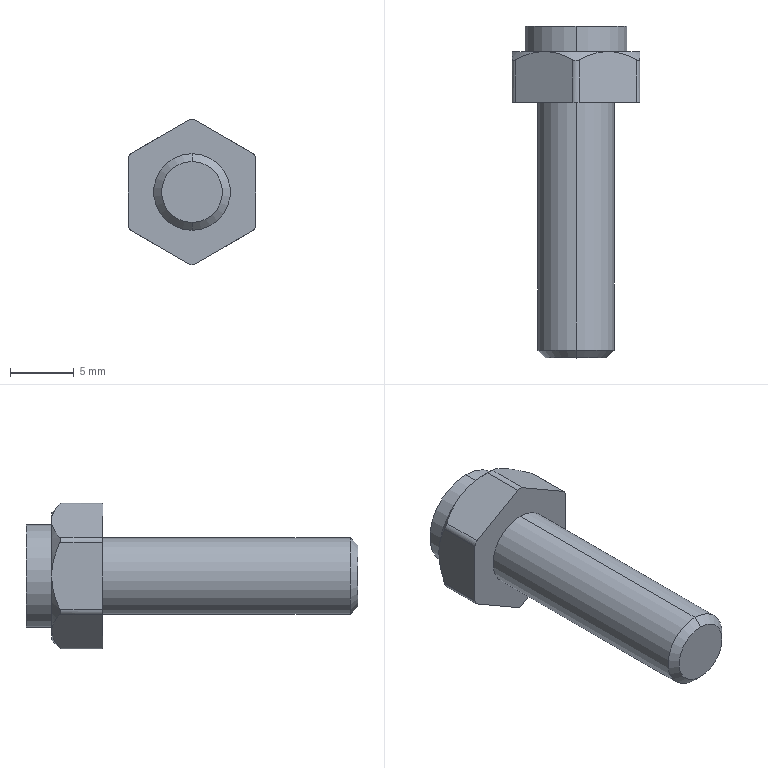Part | STEP file | _TDB86-M6-L20-001 | 1 solid | 30 faces | box 10 x 26 x 11.392 mm | volume 1007 mm3 | cylinder 11 | plane 10 | cone 9 | commonest cylinder face diameters 1 x7 6 x2 8 x2